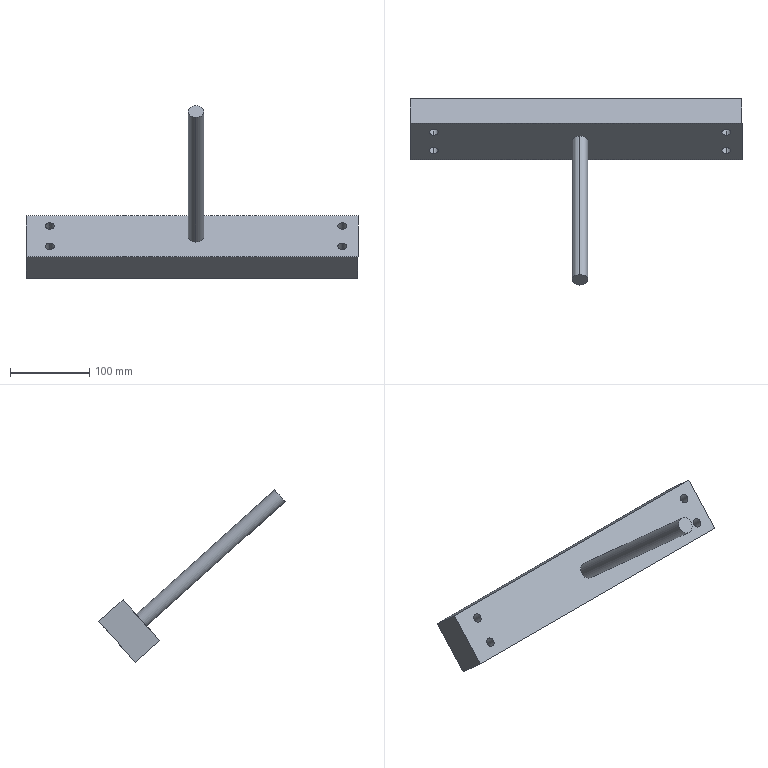Part | Creo | 1 solid | 30 faces | box 418.804 x 235.019 x 217.594 mm | volume 1236938 mm3 | cylinder 18 | plane 12 | commonest cylinder face diameters 11 x8 17.25 x8 20 x2
STEP:
#1=CARTESIAN_POINT('',(0.,0.,0.));
#2=DIRECTION('',(0.,0.,1.));
#3=DIRECTION('',(1.,0.,0.));
#4=AXIS2_PLACEMENT_3D('',#1,#2,#3);
#5=CARTESIAN_POINT('',(5.524,278.128,205.97));
#6=VERTEX_POINT('',#5);
#7=CARTESIAN_POINT('',(5.524,264.758,191.095));
#8=VERTEX_POINT('',#7);
#9=CARTESIAN_POINT('',(5.524,271.443,198.533));
#10=DIRECTION('',(0.000000011,-0.7437,0.6685));
#11=DIRECTION('',(-0.000000021,0.6685,0.7437));
#12=AXIS2_PLACEMENT_3D('',#9,#10,#11);
#13=CIRCLE('',#12,10.);
#14=EDGE_CURVE('',#6,#8,#13,.T.);
#15=ORIENTED_EDGE('',*,*,#14,.F.);
#16=CARTESIAN_POINT('',(5.524,271.443,198.533));
#17=DIRECTION('',(0.000000011,-0.7437,0.6685));
#18=DIRECTION('',(0.,-0.6685,-0.7437));
#19=AXIS2_PLACEMENT_3D('',#16,#17,#18);
#20=CIRCLE('',#19,10.);
#21=EDGE_CURVE('',#8,#6,#20,.T.);
#22=ORIENTED_EDGE('',*,*,#21,.F.);
#23=EDGE_LOOP('',(#15,#22));
#24=FACE_OUTER_BOUND('',#23,.F.);
#25=CARTESIAN_POINT('',(5.524,271.443,198.533));
#26=DIRECTION('',(-0.000000011,0.7437,-0.6685));
#27=DIRECTION('',(0.,0.6685,0.7437));
#28=AXIS2_PLACEMENT_3D('',#25,#26,#27);
#29=PLANE('',#28);
#30=ADVANCED_FACE('',(#24),#29,.F.);
#31=ORIENTED_EDGE('',*,*,#14,.T.);
#32=CARTESIAN_POINT('',(5.524,439.537,34.005));
#33=VERTEX_POINT('',#32);
#34=CARTESIAN_POINT('',(5.524,264.758,191.095));
#35=DIRECTION('',(-0.000000011,0.7437,-0.6685));
#36=VECTOR('',#35,235.);
#37=LINE('',#34,#36);
#38=EDGE_CURVE('',#8,#33,#37,.T.);
#39=ORIENTED_EDGE('',*,*,#38,.T.);
#40=CARTESIAN_POINT('',(5.524,452.906,48.88));
#41=VERTEX_POINT('',#40);
#42=CARTESIAN_POINT('',(5.524,446.222,41.442));
#43=DIRECTION('',(-0.000000011,0.7437,-0.6685));
#44=DIRECTION('',(0.000000021,-0.6685,-0.7437));
#45=AXIS2_PLACEMENT_3D('',#42,#43,#44);
#46=CIRCLE('',#45,10.);
#47=EDGE_CURVE('',#33,#41,#46,.T.);
#48=ORIENTED_EDGE('',*,*,#47,.T.);
#49=CARTESIAN_POINT('',(5.524,278.128,205.97));
#50=DIRECTION('',(-0.000000011,0.7437,-0.6685));
#51=VECTOR('',#50,235.);
#52=LINE('',#49,#51);
#53=EDGE_CURVE('',#6,#41,#52,.T.);
#54=ORIENTED_EDGE('',*,*,#53,.F.);
#55=EDGE_LOOP('',(#31,#39,#48,#54));
#56=FACE_OUTER_BOUND('',#55,.F.);
#57=CARTESIAN_POINT('',(5.524,327.223,148.398));
#58=DIRECTION('',(-0.000000011,0.7437,-0.6685));
#59=DIRECTION('',(0.,0.6685,0.7437));
#60=AXIS2_PLACEMENT_3D('',#57,#58,#59);
#61=CYLINDRICAL_SURFACE('',#60,10.);
#62=ADVANCED_FACE('',(#56),#61,.T.);
#63=ORIENTED_EDGE('',*,*,#21,.T.);
#64=ORIENTED_EDGE('',*,*,#53,.T.);
#65=CARTESIAN_POINT('',(5.524,446.222,41.442));
#66=DIRECTION('',(-0.000000011,0.7437,-0.6685));
#67=DIRECTION('',(-0.000000011,0.6685,0.7437));
#68=AXIS2_PLACEMENT_3D('',#65,#66,#67);
#69=CIRCLE('',#68,10.);
#70=EDGE_CURVE('',#41,#33,#69,.T.);
#71=ORIENTED_EDGE('',*,*,#70,.T.);
#72=ORIENTED_EDGE('',*,*,#38,.F.);
#73=EDGE_LOOP('',(#63,#64,#71,#72));
#74=FACE_OUTER_BOUND('',#73,.F.);
#75=CARTESIAN_POINT('',(5.524,327.223,148.398));
#76=DIRECTION('',(-0.000000011,0.7437,-0.6685));
#77=DIRECTION('',(0.,0.6685,0.7437));
#78=AXIS2_PLACEMENT_3D('',#75,#76,#77);
#79=CYLINDRICAL_SURFACE('',#78,10.);
#80=ADVANCED_FACE('',(#74),#79,.T.);
#81=CARTESIAN_POINT('',(209.927,469.284,67.101));
#82=VERTEX_POINT('',#81);
#83=CARTESIAN_POINT('',(209.927,423.159,15.783));
#84=VERTEX_POINT('',#83);
#85=CARTESIAN_POINT('',(209.927,469.284,67.101));
#86=DIRECTION('',(0.,-0.6685,-0.7437));
#87=VECTOR('',#86,69.);
#88=LINE('',#85,#87);
#89=EDGE_CURVE('',#82,#84,#88,.T.);
#90=ORIENTED_EDGE('',*,*,#89,.T.);
#91=CARTESIAN_POINT('',(-208.878,423.159,15.783));
#92=VERTEX_POINT('',#91);
#93=CARTESIAN_POINT('',(-208.878,423.159,15.783));
#94=DIRECTION('',(1.,0.000000025,0.000000011));
#95=VECTOR('',#94,418.804);
#96=LINE('',#93,#95);
#97=EDGE_CURVE('',#92,#84,#96,.T.);
#98=ORIENTED_EDGE('',*,*,#97,.F.);
#99=CARTESIAN_POINT('',(-208.878,469.284,67.101));
#100=VERTEX_POINT('',#99);
#101=CARTESIAN_POINT('',(-208.878,423.159,15.783));
#102=DIRECTION('',(0.,0.6685,0.7437));
#103=VECTOR('',#102,69.);
#104=LINE('',#101,#103);
#105=EDGE_CURVE('',#92,#100,#104,.T.);
#106=ORIENTED_EDGE('',*,*,#105,.T.);
#107=CARTESIAN_POINT('',(209.927,469.284,67.101));
#108=DIRECTION('',(-1.,-0.000000025,-0.000000011));
#109=VECTOR('',#108,418.804);
#110=LINE('',#107,#109);
#111=EDGE_CURVE('',#82,#100,#110,.T.);
#112=ORIENTED_EDGE('',*,*,#111,.F.);
#113=EDGE_LOOP('',(#90,#98,#106,#112));
#114=FACE_OUTER_BOUND('',#113,.F.);
#115=CARTESIAN_POINT('',(-173.378,457.753,54.272));
#116=VERTEX_POINT('',#115);
#117=CARTESIAN_POINT('',(-178.878,454.076,50.181));
#118=VERTEX_POINT('',#117);
#119=CARTESIAN_POINT('',(-178.878,457.753,54.272));
#120=DIRECTION('',(-0.000000011,0.7437,-0.6685));
#121=DIRECTION('',(1.,0.000000015,0.));
#122=AXIS2_PLACEMENT_3D('',#119,#120,#121);
#123=CIRCLE('',#122,5.5);
#124=EDGE_CURVE('',#116,#118,#123,.T.);
#125=ORIENTED_EDGE('',*,*,#124,.F.);
#126=CARTESIAN_POINT('',(-178.878,461.429,58.362));
#127=VERTEX_POINT('',#126);
#128=CARTESIAN_POINT('',(-178.878,457.753,54.272));
#129=DIRECTION('',(-0.000000011,0.7437,-0.6685));
#130=DIRECTION('',(0.,0.6685,0.7437));
#131=AXIS2_PLACEMENT_3D('',#128,#129,#130);
#132=CIRCLE('',#131,5.5);
#133=EDGE_CURVE('',#127,#116,#132,.T.);
#134=ORIENTED_EDGE('',*,*,#133,.F.);
#135=CARTESIAN_POINT('',(-178.878,457.753,54.272));
#136=DIRECTION('',(-0.000000011,0.7437,-0.6685));
#137=DIRECTION('',(0.,-0.6685,-0.7437));
#138=AXIS2_PLACEMENT_3D('',#135,#136,#137);
#139=CIRCLE('',#138,5.5);
#140=EDGE_CURVE('',#118,#127,#139,.T.);
#141=ORIENTED_EDGE('',*,*,#140,.F.);
#142=EDGE_LOOP('',(#125,#134,#141));
#143=FACE_BOUND('',#142,.F.);
#144=CARTESIAN_POINT('',(195.427,434.691,28.613));
#145=VERTEX_POINT('',#144);
#146=CARTESIAN_POINT('',(189.927,431.014,24.522));
#147=VERTEX_POINT('',#146);
#148=CARTESIAN_POINT('',(189.927,434.691,28.613));
#149=DIRECTION('',(-0.000000011,0.7437,-0.6685));
#150=DIRECTION('',(1.,0.000000015,0.));
#151=AXIS2_PLACEMENT_3D('',#148,#149,#150);
#152=CIRCLE('',#151,5.5);
#153=EDGE_CURVE('',#145,#147,#152,.T.);
#154=ORIENTED_EDGE('',*,*,#153,.F.);
#155=CARTESIAN_POINT('',(189.927,438.367,32.703));
#156=VERTEX_POINT('',#155);
#157=CARTESIAN_POINT('',(189.927,434.691,28.613));
#158=DIRECTION('',(-0.000000011,0.7437,-0.6685));
#159=DIRECTION('',(0.,0.6685,0.7437));
#160=AXIS2_PLACEMENT_3D('',#157,#158,#159);
#161=CIRCLE('',#160,5.5);
#162=EDGE_CURVE('',#156,#145,#161,.T.);
#163=ORIENTED_EDGE('',*,*,#162,.F.);
#164=CARTESIAN_POINT('',(189.927,434.691,28.613));
#165=DIRECTION('',(-0.000000011,0.7437,-0.6685));
#166=DIRECTION('',(0.,-0.6685,-0.7437));
#167=AXIS2_PLACEMENT_3D('',#164,#165,#166);
#168=CIRCLE('',#167,5.5);
#169=EDGE_CURVE('',#147,#156,#168,.T.);
#170=ORIENTED_EDGE('',*,*,#169,.F.);
#171=EDGE_LOOP('',(#154,#163,#170));
#172=FACE_BOUND('',#171,.F.);
#173=CARTESIAN_POINT('',(195.427,457.753,54.272));
#174=VERTEX_POINT('',#173);
#175=CARTESIAN_POINT('',(189.927,454.076,50.181));
#176=VERTEX_POINT('',#175);
#177=CARTESIAN_POINT('',(189.927,457.753,54.272));
#178=DIRECTION('',(-0.000000011,0.7437,-0.6685));
#179=DIRECTION('',(1.,0.000000015,0.));
#180=AXIS2_PLACEMENT_3D('',#177,#178,#179);
#181=CIRCLE('',#180,5.5);
#182=EDGE_CURVE('',#174,#176,#181,.T.);
#183=ORIENTED_EDGE('',*,*,#182,.F.);
#184=CARTESIAN_POINT('',(189.927,461.429,58.362));
#185=VERTEX_POINT('',#184);
#186=CARTESIAN_POINT('',(189.927,457.753,54.272));
#187=DIRECTION('',(-0.000000011,0.7437,-0.6685));
#188=DIRECTION('',(0.,0.6685,0.7437));
#189=AXIS2_PLACEMENT_3D('',#186,#187,#188);
#190=CIRCLE('',#189,5.5);
#191=EDGE_CURVE('',#185,#174,#190,.T.);
#192=ORIENTED_EDGE('',*,*,#191,.F.);
#193=CARTESIAN_POINT('',(189.927,457.753,54.272));
#194=DIRECTION('',(-0.000000011,0.7437,-0.6685));
#195=DIRECTION('',(0.,-0.6685,-0.7437));
#196=AXIS2_PLACEMENT_3D('',#193,#194,#195);
#197=CIRCLE('',#196,5.5);
#198=EDGE_CURVE('',#176,#185,#197,.T.);
#199=ORIENTED_EDGE('',*,*,#198,.F.);
#200=EDGE_LOOP('',(#183,#192,#199));
#201=FACE_BOUND('',#200,.F.);
#202=CARTESIAN_POINT('',(-173.378,434.691,28.613));
#203=VERTEX_POINT('',#202);
#204=CARTESIAN_POINT('',(-178.878,431.014,24.522));
#205=VERTEX_POINT('',#204);
#206=CARTESIAN_POINT('',(-178.878,434.691,28.613));
#207=DIRECTION('',(-0.000000011,0.7437,-0.6685));
#208=DIRECTION('',(1.,0.000000015,0.));
#209=AXIS2_PLACEMENT_3D('',#206,#207,#208);
#210=CIRCLE('',#209,5.5);
#211=EDGE_CURVE('',#203,#205,#210,.T.);
#212=ORIENTED_EDGE('',*,*,#211,.F.);
#213=CARTESIAN_POINT('',(-178.878,438.367,32.703));
#214=VERTEX_POINT('',#213);
#215=CARTESIAN_POINT('',(-178.878,434.691,28.613));
#216=DIRECTION('',(-0.000000011,0.7437,-0.6685));
#217=DIRECTION('',(0.,0.6685,0.7437));
#218=AXIS2_PLACEMENT_3D('',#215,#216,#217);
#219=CIRCLE('',#218,5.5);
#220=EDGE_CURVE('',#214,#203,#219,.T.);
#221=ORIENTED_EDGE('',*,*,#220,.F.);
#222=CARTESIAN_POINT('',(-178.878,434.691,28.613));
#223=DIRECTION('',(-0.000000011,0.7437,-0.6685));
#224=DIRECTION('',(0.,-0.6685,-0.7437));
#225=AXIS2_PLACEMENT_3D('',#222,#223,#224);
#226=CIRCLE('',#225,5.5);
#227=EDGE_CURVE('',#205,#214,#226,.T.);
#228=ORIENTED_EDGE('',*,*,#227,.F.);
#229=EDGE_LOOP('',(#212,#221,#228));
#230=FACE_BOUND('',#229,.F.);
#231=ORIENTED_EDGE('',*,*,#47,.F.);
#232=ORIENTED_EDGE('',*,*,#70,.F.);
#233=EDGE_LOOP('',(#231,#232));
#234=FACE_BOUND('',#233,.F.);
#235=CARTESIAN_POINT('',(-53.476,423.159,15.783));
#236=DIRECTION('',(0.000000011,-0.7437,0.6685));
#237=DIRECTION('',(0.,-0.6685,-0.7437));
#238=AXIS2_PLACEMENT_3D('',#235,#236,#237);
#239=PLANE('',#238);
#240=ADVANCED_FACE('',(#114,#143,#172,#201,#230,#234),#239,.T.);
#241=ORIENTED_EDGE('',*,*,#220,.T.);
#242=ORIENTED_EDGE('',*,*,#211,.T.);
#243=CARTESIAN_POINT('',(-178.878,453.326,4.468));
#244=VERTEX_POINT('',#243);
#245=CARTESIAN_POINT('',(-178.878,453.326,4.468));
#246=DIRECTION('',(0.000000011,-0.7437,0.6685));
#247=VECTOR('',#246,30.);
#248=LINE('',#245,#247);
#249=EDGE_CURVE('',#244,#205,#248,.T.);
#250=ORIENTED_EDGE('',*,*,#249,.F.);
#251=CARTESIAN_POINT('',(-173.378,457.003,8.559));
#252=VERTEX_POINT('',#251);
#253=CARTESIAN_POINT('',(-178.878,457.003,8.559));
#254=DIRECTION('',(0.000000011,-0.7437,0.6685));
#255=DIRECTION('',(0.,-0.6685,-0.7437));
#256=AXIS2_PLACEMENT_3D('',#253,#254,#255);
#257=CIRCLE('',#256,5.5);
#258=EDGE_CURVE('',#244,#252,#257,.T.);
#259=ORIENTED_EDGE('',*,*,#258,.T.);
#260=CARTESIAN_POINT('',(-178.878,460.679,12.649));
#261=VERTEX_POINT('',#260);
#262=CARTESIAN_POINT('',(-178.878,457.003,8.559));
#263=DIRECTION('',(0.000000011,-0.7437,0.6685));
#264=DIRECTION('',(1.,0.000000015,0.));
#265=AXIS2_PLACEMENT_3D('',#262,#263,#264);
#266=CIRCLE('',#265,5.5);
#267=EDGE_CURVE('',#252,#261,#266,.T.);
#268=ORIENTED_EDGE('',*,*,#267,.T.);
#269=CARTESIAN_POINT('',(-178.878,460.679,12.649));
#270=DIRECTION('',(0.000000011,-0.7437,0.6685));
#271=VECTOR('',#270,30.);
#272=LINE('',#269,#271);
#273=EDGE_CURVE('',#261,#214,#272,.T.);
#274=ORIENTED_EDGE('',*,*,#273,.T.);
#275=EDGE_LOOP('',(#241,#242,#250,#259,#268,#274));
#276=FACE_OUTER_BOUND('',#275,.F.);
#277=CARTESIAN_POINT('',(-178.878,457.003,8.559));
#278=DIRECTION('',(0.000000011,-0.7437,0.6685));
#279=DIRECTION('',(0.,-0.6685,-0.7437));
#280=AXIS2_PLACEMENT_3D('',#277,#278,#279);
#281=CYLINDRICAL_SURFACE('',#280,5.5);
#282=ADVANCED_FACE('',(#276),#281,.F.);
#283=ORIENTED_EDGE('',*,*,#227,.T.);
#284=ORIENTED_EDGE('',*,*,#273,.F.);
#285=CARTESIAN_POINT('',(-184.378,457.003,8.559));
#286=VERTEX_POINT('',#285);
#287=CARTESIAN_POINT('',(-178.878,457.003,8.559));
#288=DIRECTION('',(0.000000011,-0.7437,0.6685));
#289=DIRECTION('',(0.,0.6685,0.7437));
#290=AXIS2_PLACEMENT_3D('',#287,#288,#289);
#291=CIRCLE('',#290,5.5);
#292=EDGE_CURVE('',#261,#286,#291,.T.);
#293=ORIENTED_EDGE('',*,*,#292,.T.);
#294=CARTESIAN_POINT('',(-178.878,457.003,8.559));
#295=DIRECTION('',(0.000000011,-0.7437,0.6685));
#296=DIRECTION('',(-1.,-0.000000015,0.));
#297=AXIS2_PLACEMENT_3D('',#294,#295,#296);
#298=CIRCLE('',#297,5.5);
#299=EDGE_CURVE('',#286,#244,#298,.T.);
#300=ORIENTED_EDGE('',*,*,#299,.T.);
#301=ORIENTED_EDGE('',*,*,#249,.T.);
#302=EDGE_LOOP('',(#283,#284,#293,#300,#301));
#303=FACE_OUTER_BOUND('',#302,.F.);
#304=CARTESIAN_POINT('',(-178.878,457.003,8.559));
#305=DIRECTION('',(0.000000011,-0.7437,0.6685));
#306=DIRECTION('',(0.,-0.6685,-0.7437));
#307=AXIS2_PLACEMENT_3D('',#304,#305,#306);
#308=CYLINDRICAL_SURFACE('',#307,5.5);
#309=ADVANCED_FACE('',(#303),#308,.F.);
#310=CARTESIAN_POINT('',(-187.503,457.003,8.559));
#311=VERTEX_POINT('',#310);
#312=CARTESIAN_POINT('',(-178.878,462.768,14.973));
#313=VERTEX_POINT('',#312);
#314=CARTESIAN_POINT('',(-178.878,457.003,8.559));
#315=DIRECTION('',(-0.000000011,0.7437,-0.6685));
#316=DIRECTION('',(-1.,-0.000000015,0.));
#317=AXIS2_PLACEMENT_3D('',#314,#315,#316);
#318=CIRCLE('',#317,8.625);
#319=EDGE_CURVE('',#311,#313,#318,.T.);
#320=ORIENTED_EDGE('',*,*,#319,.F.);
#321=CARTESIAN_POINT('',(-178.878,451.237,2.144));
#322=VERTEX_POINT('',#321);
#323=CARTESIAN_POINT('',(-178.878,457.003,8.559));
#324=DIRECTION('',(-0.000000011,0.7437,-0.6685));
#325=DIRECTION('',(0.,-0.6685,-0.7437));
#326=AXIS2_PLACEMENT_3D('',#323,#324,#325);
#327=CIRCLE('',#326,8.625);
#328=EDGE_CURVE('',#322,#311,#327,.T.);
#329=ORIENTED_EDGE('',*,*,#328,.F.);
#330=CARTESIAN_POINT('',(-170.253,457.003,8.559));
#331=VERTEX_POINT('',#330);
#332=CARTESIAN_POINT('',(-178.878,457.003,8.559));
#333=DIRECTION('',(-0.000000011,0.7437,-0.6685));
#334=DIRECTION('',(1.,0.000000015,0.));
#335=AXIS2_PLACEMENT_3D('',#332,#333,#334);
#336=CIRCLE('',#335,8.625);
#337=EDGE_CURVE('',#331,#322,#336,.T.);
#338=ORIENTED_EDGE('',*,*,#337,.F.);
#339=CARTESIAN_POINT('',(-178.878,457.003,8.559));
#340=DIRECTION('',(-0.000000011,0.7437,-0.6685));
#341=DIRECTION('',(0.,0.6685,0.7437));
#342=AXIS2_PLACEMENT_3D('',#339,#340,#341);
#343=CIRCLE('',#342,8.625);
#344=EDGE_CURVE('',#313,#331,#343,.T.);
#345=ORIENTED_EDGE('',*,*,#344,.F.);
#346=EDGE_LOOP('',(#320,#329,#338,#345));
#347=FACE_OUTER_BOUND('',#346,.F.);
#348=ORIENTED_EDGE('',*,*,#267,.F.);
#349=ORIENTED_EDGE('',*,*,#258,.F.);
#350=ORIENTED_EDGE('',*,*,#299,.F.);
#351=ORIENTED_EDGE('',*,*,#292,.F.);
#352=EDGE_LOOP('',(#348,#349,#350,#351));
#353=FACE_BOUND('',#352,.F.);
#354=CARTESIAN_POINT('',(-178.878,457.003,8.559));
#355=DIRECTION('',(0.000000011,-0.7437,0.6685));
#356=DIRECTION('',(0.,-0.6685,-0.7437));
#357=AXIS2_PLACEMENT_3D('',#354,#355,#356);
#358=PLANE('',#357);
#359=ADVANCED_FACE('',(#347,#353),#358,.F.);
#360=CARTESIAN_POINT('',(-178.878,470.949,7.62));
#361=VERTEX_POINT('',#360);
#362=CARTESIAN_POINT('',(-187.503,465.184,1.206));
#363=VERTEX_POINT('',#362);
#364=CARTESIAN_POINT('',(-178.878,465.184,1.206));
#365=DIRECTION('',(0.000000011,-0.7437,0.6685));
#366=DIRECTION('',(0.,0.6685,0.7437));
#367=AXIS2_PLACEMENT_3D('',#364,#365,#366);
#368=CIRCLE('',#367,8.625);
#369=EDGE_CURVE('',#361,#363,#368,.T.);
#370=ORIENTED_EDGE('',*,*,#369,.T.);
#371=CARTESIAN_POINT('',(-178.878,459.418,-5.209));
#372=VERTEX_POINT('',#371);
#373=CARTESIAN_POINT('',(-178.878,465.184,1.206));
#374=DIRECTION('',(0.000000011,-0.7437,0.6685));
#375=DIRECTION('',(-1.,-0.000000015,0.));
#376=AXIS2_PLACEMENT_3D('',#373,#374,#375);
#377=CIRCLE('',#376,8.625);
#378=EDGE_CURVE('',#363,#372,#377,.T.);
#379=ORIENTED_EDGE('',*,*,#378,.T.);
#380=CARTESIAN_POINT('',(-178.878,451.237,2.144));
#381=DIRECTION('',(-0.000000011,0.7437,-0.6685));
#382=VECTOR('',#381,11.);
#383=LINE('',#380,#382);
#384=EDGE_CURVE('',#322,#372,#383,.T.);
#385=ORIENTED_EDGE('',*,*,#384,.F.);
#386=ORIENTED_EDGE('',*,*,#328,.T.);
#387=ORIENTED_EDGE('',*,*,#319,.T.);
#388=CARTESIAN_POINT('',(-178.878,462.768,14.973));
#389=DIRECTION('',(-0.000000011,0.7437,-0.6685));
#390=VECTOR('',#389,11.);
#391=LINE('',#388,#390);
#392=EDGE_CURVE('',#313,#361,#391,.T.);
#393=ORIENTED_EDGE('',*,*,#392,.T.);
#394=EDGE_LOOP('',(#370,#379,#385,#386,#387,#393));
#395=FACE_OUTER_BOUND('',#394,.F.);
#396=CARTESIAN_POINT('',(-178.878,457.003,8.559));
#397=DIRECTION('',(-0.000000011,0.7437,-0.6685));
#398=DIRECTION('',(0.,0.6685,0.7437));
#399=AXIS2_PLACEMENT_3D('',#396,#397,#398);
#400=CYLINDRICAL_SURFACE('',#399,8.625);
#401=ADVANCED_FACE('',(#395),#400,.F.);
#402=CARTESIAN_POINT('',(209.927,499.777,39.694));
#403=VERTEX_POINT('',#402);
#404=CARTESIAN_POINT('',(-208.878,499.777,39.694));
#405=VERTEX_POINT('',#404);
#406=CARTESIAN_POINT('',(209.927,499.777,39.694));
#407=DIRECTION('',(-1.,-0.000000025,-0.000000011));
#408=VECTOR('',#407,418.804);
#409=LINE('',#406,#408);
#410=EDGE_CURVE('',#403,#405,#409,.T.);
#411=ORIENTED_EDGE('',*,*,#410,.T.);
#412=CARTESIAN_POINT('',(-208.878,453.653,-11.624));
#413=VERTEX_POINT('',#412);
#414=CARTESIAN_POINT('',(-208.878,499.777,39.694));
#415=DIRECTION('',(0.,-0.6685,-0.7437));
#416=VECTOR('',#415,69.);
#417=LINE('',#414,#416);
#418=EDGE_CURVE('',#405,#413,#417,.T.);
#419=ORIENTED_EDGE('',*,*,#418,.T.);
#420=CARTESIAN_POINT('',(209.927,453.653,-11.624));
#421=VERTEX_POINT('',#420);
#422=CARTESIAN_POINT('',(-208.878,453.653,-11.624));
#423=DIRECTION('',(1.,0.000000025,0.000000011));
#424=VECTOR('',#423,418.804);
#425=LINE('',#422,#424);
#426=EDGE_CURVE('',#413,#421,#425,.T.);
#427=ORIENTED_EDGE('',*,*,#426,.T.);
#428=CARTESIAN_POINT('',(209.927,453.653,-11.624));
#429=DIRECTION('',(0.,0.6685,0.7437));
#430=VECTOR('',#429,69.);
#431=LINE('',#428,#430);
#432=EDGE_CURVE('',#421,#403,#431,.T.);
#433=ORIENTED_EDGE('',*,*,#432,.T.);
#434=EDGE_LOOP('',(#411,#419,#427,#433));
#435=FACE_OUTER_BOUND('',#434,.F.);
#436=CARTESIAN_POINT('',(181.302,488.246,26.865));
#437=VERTEX_POINT('',#436);
#438=CARTESIAN_POINT('',(189.927,482.481,20.45));
#439=VERTEX_POINT('',#438);
#440=CARTESIAN_POINT('',(189.927,488.246,26.865));
#441=DIRECTION('',(0.000000011,-0.7437,0.6685));
#442=DIRECTION('',(-1.,-0.000000015,0.));
#443=AXIS2_PLACEMENT_3D('',#440,#441,#442);
#444=CIRCLE('',#443,8.625);
#445=EDGE_CURVE('',#437,#439,#444,.T.);
#446=ORIENTED_EDGE('',*,*,#445,.F.);
#447=CARTESIAN_POINT('',(189.927,494.012,33.279));
#448=VERTEX_POINT('',#447);
#449=CARTESIAN_POINT('',(189.927,488.246,26.865));
#450=DIRECTION('',(0.000000011,-0.7437,0.6685));
#451=DIRECTION('',(0.,0.6685,0.7437));
#452=AXIS2_PLACEMENT_3D('',#449,#450,#451);
#453=CIRCLE('',#452,8.625);
#454=EDGE_CURVE('',#448,#437,#453,.T.);
#455=ORIENTED_EDGE('',*,*,#454,.F.);
#456=CARTESIAN_POINT('',(189.927,488.246,26.865));
#457=DIRECTION('',(0.000000011,-0.7437,0.6685));
#458=DIRECTION('',(0.,-0.6685,-0.7437));
#459=AXIS2_PLACEMENT_3D('',#456,#457,#458);
#460=CIRCLE('',#459,8.625);
#461=EDGE_CURVE('',#439,#448,#460,.T.);
#462=ORIENTED_EDGE('',*,*,#461,.F.);
#463=EDGE_LOOP('',(#446,#455,#462));
#464=FACE_BOUND('',#463,.F.);
#465=CARTESIAN_POINT('',(30.024,454.99,-10.137));
#466=VERTEX_POINT('',#465);
#467=CARTESIAN_POINT('',(-18.976,454.99,-10.137));
#468=VERTEX_POINT('',#467);
#469=CARTESIAN_POINT('',(30.024,454.99,-10.137));
#470=DIRECTION('',(-1.,-0.000000021,-0.000000007));
#471=VECTOR('',#470,49.);
#472=LINE('',#469,#471);
#473=EDGE_CURVE('',#466,#468,#472,.T.);
#474=ORIENTED_EDGE('',*,*,#473,.T.);
#475=CARTESIAN_POINT('',(-26.976,460.337,-4.187));
#476=VERTEX_POINT('',#475);
#477=CARTESIAN_POINT('',(-18.976,454.99,-10.137));
#478=CARTESIAN_POINT('',(-19.692,454.992,-10.134));
#479=CARTESIAN_POINT('',(-21.07,455.113,-10.));
#480=CARTESIAN_POINT('',(-23.028,455.655,-9.396));
#481=CARTESIAN_POINT('',(-24.696,456.513,-8.442));
#482=CARTESIAN_POINT('',(-25.98,457.629,-7.201));
#483=CARTESIAN_POINT('',(-26.792,458.938,-5.744));
#484=CARTESIAN_POINT('',(-26.972,459.858,-4.72));
#485=CARTESIAN_POINT('',(-26.976,460.337,-4.187));
#486=B_SPLINE_CURVE_WITH_KNOTS('',3,(#477,#478,#479,#480,#481,#482,#483,#484,#485),.UNSPECIFIED.,.F.,.F.,(4,1,1,1,1,1,4),(0.,0.1667,0.3333,0.5,0.6667,0.8333,1.),.UNSPECIFIED.);
#487=EDGE_CURVE('',#468,#476,#486,.T.);
#488=ORIENTED_EDGE('',*,*,#487,.T.);
#489=CARTESIAN_POINT('',(-26.976,493.092,32.257));
#490=VERTEX_POINT('',#489);
#491=CARTESIAN_POINT('',(-26.976,460.337,-4.187));
#492=DIRECTION('',(-0.000000019,0.6685,0.7437));
#493=VECTOR('',#492,49.);
#494=LINE('',#491,#493);
#495=EDGE_CURVE('',#476,#490,#494,.T.);
#496=ORIENTED_EDGE('',*,*,#495,.T.);
#497=CARTESIAN_POINT('',(-18.976,498.44,38.207));
#498=VERTEX_POINT('',#497);
#499=CARTESIAN_POINT('',(-26.972,493.572,32.79));
#500=CARTESIAN_POINT('',(-26.792,494.492,33.814));
#501=CARTESIAN_POINT('',(-25.98,495.801,35.27));
#502=CARTESIAN_POINT('',(-24.697,496.917,36.511));
#503=CARTESIAN_POINT('',(-23.028,497.775,37.466));
#504=CARTESIAN_POINT('',(-21.07,498.317,38.07));
#505=CARTESIAN_POINT('',(-19.692,498.438,38.204));
#506=CARTESIAN_POINT('',(-18.976,498.44,38.207));
#507=B_SPLINE_CURVE_WITH_KNOTS('',3,(#489,#499,#500,#501,#502,#503,#504,#505,#506),.UNSPECIFIED.,.F.,.F.,(4,1,1,1,1,1,4),(0.,0.1667,0.3333,0.5,0.6667,0.8333,1.),.UNSPECIFIED.);
#508=EDGE_CURVE('',#490,#498,#507,.T.);
#509=ORIENTED_EDGE('',*,*,#508,.T.);
#510=CARTESIAN_POINT('',(30.024,498.44,38.207));
#511=VERTEX_POINT('',#510);
#512=CARTESIAN_POINT('',(-18.976,498.44,38.207));
#513=DIRECTION('',(1.,0.000000021,0.000000007));
#514=VECTOR('',#513,49.);
#515=LINE('',#512,#514);
#516=EDGE_CURVE('',#498,#511,#515,.T.);
#517=ORIENTED_EDGE('',*,*,#516,.T.);
#518=CARTESIAN_POINT('',(38.024,493.092,32.257));
#519=VERTEX_POINT('',#518);
#520=CARTESIAN_POINT('',(30.741,498.438,38.204));
#521=CARTESIAN_POINT('',(32.118,498.317,38.07));
#522=CARTESIAN_POINT('',(34.077,497.775,37.466));
#523=CARTESIAN_POINT('',(35.745,496.917,36.512));
#524=CARTESIAN_POINT('',(37.029,495.801,35.271));
#525=CARTESIAN_POINT('',(37.841,494.492,33.814));
#526=CARTESIAN_POINT('',(38.021,493.572,32.79));
#527=CARTESIAN_POINT('',(38.024,493.092,32.257));
#528=B_SPLINE_CURVE_WITH_KNOTS('',3,(#510,#520,#521,#522,#523,#524,#525,#526,#527),.UNSPECIFIED.,.F.,.F.,(4,1,1,1,1,1,4),(0.,0.1667,0.3333,0.5,0.6667,0.8333,1.),.UNSPECIFIED.);
#529=EDGE_CURVE('',#511,#519,#528,.T.);
#530=ORIENTED_EDGE('',*,*,#529,.T.);
#531=CARTESIAN_POINT('',(38.024,460.337,-4.187));
#532=VERTEX_POINT('',#531);
#533=CARTESIAN_POINT('',(38.024,493.092,32.257));
#534=DIRECTION('',(0.000000013,-0.6685,-0.7437));
#535=VECTOR('',#534,49.);
#536=LINE('',#533,#535);
#537=EDGE_CURVE('',#519,#532,#536,.T.);
#538=ORIENTED_EDGE('',*,*,#537,.T.);
#539=CARTESIAN_POINT('',(38.021,459.858,-4.72));
#540=CARTESIAN_POINT('',(37.841,458.938,-5.744));
#541=CARTESIAN_POINT('',(37.029,457.629,-7.2));
#542=CARTESIAN_POINT('',(35.746,456.513,-8.441));
#543=CARTESIAN_POINT('',(34.077,455.655,-9.396));
#544=CARTESIAN_POINT('',(32.119,455.113,-10.));
#545=CARTESIAN_POINT('',(30.741,454.992,-10.134));
#546=CARTESIAN_POINT('',(30.024,454.99,-10.137));
#547=B_SPLINE_CURVE_WITH_KNOTS('',3,(#531,#539,#540,#541,#542,#543,#544,#545,#546),.UNSPECIFIED.,.F.,.F.,(4,1,1,1,1,1,4),(0.,0.1667,0.3333,0.5,0.6667,0.8333,1.),.UNSPECIFIED.);
#548=EDGE_CURVE('',#532,#466,#547,.T.);
#549=ORIENTED_EDGE('',*,*,#548,.T.);
#550=EDGE_LOOP('',(#474,#488,#496,#509,#517,#530,#538,#549));
#551=FACE_BOUND('',#550,.F.);
#552=CARTESIAN_POINT('',(-187.503,488.246,26.865));
#553=VERTEX_POINT('',#552);
#554=CARTESIAN_POINT('',(-178.878,482.481,20.45));
#555=VERTEX_POINT('',#554);
#556=CARTESIAN_POINT('',(-178.878,488.246,26.865));
#557=DIRECTION('',(0.000000011,-0.7437,0.6685));
#558=DIRECTION('',(-1.,-0.000000015,0.));
#559=AXIS2_PLACEMENT_3D('',#556,#557,#558);
#560=CIRCLE('',#559,8.625);
#561=EDGE_CURVE('',#553,#555,#560,.T.);
#562=ORIENTED_EDGE('',*,*,#561,.F.);
#563=CARTESIAN_POINT('',(-178.878,494.012,33.279));
#564=VERTEX_POINT('',#563);
#565=CARTESIAN_POINT('',(-178.878,488.246,26.865));
#566=DIRECTION('',(0.000000011,-0.7437,0.6685));
#567=DIRECTION('',(0.,0.6685,0.7437));
#568=AXIS2_PLACEMENT_3D('',#565,#566,#567);
#569=CIRCLE('',#568,8.625);
#570=EDGE_CURVE('',#564,#553,#569,.T.);
#571=ORIENTED_EDGE('',*,*,#570,.F.);
#572=CARTESIAN_POINT('',(-178.878,488.246,26.865));
#573=DIRECTION('',(0.000000011,-0.7437,0.6685));
#574=DIRECTION('',(0.,-0.6685,-0.7437));
#575=AXIS2_PLACEMENT_3D('',#572,#573,#574);
#576=CIRCLE('',#575,8.625);
#577=EDGE_CURVE('',#555,#564,#576,.T.);
#578=ORIENTED_EDGE('',*,*,#577,.F.);
#579=EDGE_LOOP('',(#562,#571,#578));
#580=FACE_BOUND('',#579,.F.);
#581=CARTESIAN_POINT('',(181.302,465.184,1.206));
#582=VERTEX_POINT('',#581);
#583=CARTESIAN_POINT('',(189.927,459.418,-5.209));
#584=VERTEX_POINT('',#583);
#585=CARTESIAN_POINT('',(189.927,465.184,1.206));
#586=DIRECTION('',(0.000000011,-0.7437,0.6685));
#587=DIRECTION('',(-1.,-0.000000015,0.));
#588=AXIS2_PLACEMENT_3D('',#585,#586,#587);
#589=CIRCLE('',#588,8.625);
#590=EDGE_CURVE('',#582,#584,#589,.T.);
#591=ORIENTED_EDGE('',*,*,#590,.F.);
#592=CARTESIAN_POINT('',(189.927,470.949,7.62));
#593=VERTEX_POINT('',#592);
#594=CARTESIAN_POINT('',(189.927,465.184,1.206));
#595=DIRECTION('',(0.000000011,-0.7437,0.6685));
#596=DIRECTION('',(0.,0.6685,0.7437));
#597=AXIS2_PLACEMENT_3D('',#594,#595,#596);
#598=CIRCLE('',#597,8.625);
#599=EDGE_CURVE('',#593,#582,#598,.T.);
#600=ORIENTED_EDGE('',*,*,#599,.F.);
#601=CARTESIAN_POINT('',(189.927,465.184,1.206));
#602=DIRECTION('',(0.000000011,-0.7437,0.6685));
#603=DIRECTION('',(0.,-0.6685,-0.7437));
#604=AXIS2_PLACEMENT_3D('',#601,#602,#603);
#605=CIRCLE('',#604,8.625);
#606=EDGE_CURVE('',#584,#593,#605,.T.);
#607=ORIENTED_EDGE('',*,*,#606,.F.);
#608=EDGE_LOOP('',(#591,#600,#607));
#609=FACE_BOUND('',#608,.F.);
#610=ORIENTED_EDGE('',*,*,#378,.F.);
#611=ORIENTED_EDGE('',*,*,#369,.F.);
#612=CARTESIAN_POINT('',(-178.878,465.184,1.206));
#613=DIRECTION('',(0.000000011,-0.7437,0.6685));
#614=DIRECTION('',(0.,-0.6685,-0.7437));
#615=AXIS2_PLACEMENT_3D('',#612,#613,#614);
#616=CIRCLE('',#615,8.625);
#617=EDGE_CURVE('',#372,#361,#616,.T.);
#618=ORIENTED_EDGE('',*,*,#617,.F.);
#619=EDGE_LOOP('',(#610,#611,#618));
#620=FACE_BOUND('',#619,.F.);
#621=CARTESIAN_POINT('',(-53.476,453.653,-11.624));
#622=DIRECTION('',(0.000000011,-0.7437,0.6685));
#623=DIRECTION('',(0.,-0.6685,-0.7437));
#624=AXIS2_PLACEMENT_3D('',#621,#622,#623);
#625=PLANE('',#624);
#626=ADVANCED_FACE('',(#435,#464,#551,#580,#609,#620),#625,.F.);
#627=ORIENTED_EDGE('',*,*,#570,.T.);
#628=ORIENTED_EDGE('',*,*,#561,.T.);
#629=CARTESIAN_POINT('',(-178.878,474.299,27.803));
#630=VERTEX_POINT('',#629);
#631=CARTESIAN_POINT('',(-178.878,474.299,27.803));
#632=DIRECTION('',(-0.000000011,0.7437,-0.6685));
#633=VECTOR('',#632,11.);
#634=LINE('',#631,#633);
#635=EDGE_CURVE('',#630,#555,#634,.T.);
#636=ORIENTED_EDGE('',*,*,#635,.F.);
#637=CARTESIAN_POINT('',(-187.503,480.065,34.218));
#638=VERTEX_POINT('',#637);
#639=CARTESIAN_POINT('',(-178.878,480.065,34.218));
#640=DIRECTION('',(-0.000000011,0.7437,-0.6685));
#641=DIRECTION('',(0.,-0.6685,-0.7437));
#642=AXIS2_PLACEMENT_3D('',#639,#640,#641);
#643=CIRCLE('',#642,8.625);
#644=EDGE_CURVE('',#630,#638,#643,.T.);
#645=ORIENTED_EDGE('',*,*,#644,.T.);
#646=CARTESIAN_POINT('',(-178.878,485.831,40.632));
#647=VERTEX_POINT('',#646);
#648=CARTESIAN_POINT('',(-178.878,480.065,34.218));
#649=DIRECTION('',(-0.000000011,0.7437,-0.6685));
#650=DIRECTION('',(-1.,-0.000000015,0.));
#651=AXIS2_PLACEMENT_3D('',#648,#649,#650);
#652=CIRCLE('',#651,8.625);
#653=EDGE_CURVE('',#638,#647,#652,.T.);
#654=ORIENTED_EDGE('',*,*,#653,.T.);
#655=CARTESIAN_POINT('',(-178.878,485.831,40.632));
#656=DIRECTION('',(-0.000000011,0.7437,-0.6685));
#657=VECTOR('',#656,11.);
#658=LINE('',#655,#657);
#659=EDGE_CURVE('',#647,#564,#658,.T.);
#660=ORIENTED_EDGE('',*,*,#659,.T.);
#661=EDGE_LOOP('',(#627,#628,#636,#645,#654,#660));
#662=FACE_OUTER_BOUND('',#661,.F.);
#663=CARTESIAN_POINT('',(-178.878,480.065,34.218));
#664=DIRECTION('',(-0.000000011,0.7437,-0.6685));
#665=DIRECTION('',(0.,0.6685,0.7437));
#666=AXIS2_PLACEMENT_3D('',#663,#664,#665);
#667=CYLINDRICAL_SURFACE('',#666,8.625);
#668=ADVANCED_FACE('',(#662),#667,.F.);
#669=ORIENTED_EDGE('',*,*,#577,.T.);
#670=ORIENTED_EDGE('',*,*,#659,.F.);
#671=CARTESIAN_POINT('',(-170.253,480.065,34.218));
#672=VERTEX_POINT('',#671);
#673=CARTESIAN_POINT('',(-178.878,480.065,34.218));
#674=DIRECTION('',(-0.000000011,0.7437,-0.6685));
#675=DIRECTION('',(0.,0.6685,0.7437));
#676=AXIS2_PLACEMENT_3D('',#673,#674,#675);
#677=CIRCLE('',#676,8.625);
#678=EDGE_CURVE('',#647,#672,#677,.T.);
#679=ORIENTED_EDGE('',*,*,#678,.T.);
#680=CARTESIAN_POINT('',(-178.878,480.065,34.218));
#681=DIRECTION('',(-0.000000011,0.7437,-0.6685));
#682=DIRECTION('',(1.,0.000000015,0.));
#683=AXIS2_PLACEMENT_3D('',#680,#681,#682);
#684=CIRCLE('',#683,8.625);
#685=EDGE_CURVE('',#672,#630,#684,.T.);
#686=ORIENTED_EDGE('',*,*,#685,.T.);
#687=ORIENTED_EDGE('',*,*,#635,.T.);
#688=EDGE_LOOP('',(#669,#670,#679,#686,#687));
#689=FACE_OUTER_BOUND('',#688,.F.);
#690=CARTESIAN_POINT('',(-178.878,480.065,34.218));
#691=DIRECTION('',(-0.000000011,0.7437,-0.6685));
#692=DIRECTION('',(0.,0.6685,0.7437));
#693=AXIS2_PLACEMENT_3D('',#690,#691,#692);
#694=CYLINDRICAL_SURFACE('',#693,8.625);
#695=ADVANCED_FACE('',(#689),#694,.F.);
#696=ORIENTED_EDGE('',*,*,#653,.F.);
#697=ORIENTED_EDGE('',*,*,#644,.F.);
#698=ORIENTED_EDGE('',*,*,#685,.F.);
#699=ORIENTED_EDGE('',*,*,#678,.F.);
#700=EDGE_LOOP('',(#696,#697,#698,#699));
#701=FACE_OUTER_BOUND('',#700,.F.);
#702=CARTESIAN_POINT('',(-173.378,480.065,34.218));
#703=VERTEX_POINT('',#702);
#704=CARTESIAN_POINT('',(-178.878,483.742,38.308));
#705=VERTEX_POINT('',#704);
#706=CARTESIAN_POINT('',(-178.878,480.065,34.218));
#707=DIRECTION('',(0.000000011,-0.7437,0.6685));
#708=DIRECTION('',(1.,0.000000015,0.));
#709=AXIS2_PLACEMENT_3D('',#706,#707,#708);
#710=CIRCLE('',#709,5.5);
#711=EDGE_CURVE('',#703,#705,#710,.T.);
#712=ORIENTED_EDGE('',*,*,#711,.F.);
#713=CARTESIAN_POINT('',(-178.878,476.388,30.127));
#714=VERTEX_POINT('',#713);
#715=CARTESIAN_POINT('',(-178.878,480.065,34.218));
#716=DIRECTION('',(0.000000011,-0.7437,0.6685));
#717=DIRECTION('',(0.,-0.6685,-0.7437));
#718=AXIS2_PLACEMENT_3D('',#715,#716,#717);
#719=CIRCLE('',#718,5.5);
#720=EDGE_CURVE('',#714,#703,#719,.T.);
#721=ORIENTED_EDGE('',*,*,#720,.F.);
#722=CARTESIAN_POINT('',(-184.378,480.065,34.218));
#723=VERTEX_POINT('',#722);
#724=CARTESIAN_POINT('',(-178.878,480.065,34.218));
#725=DIRECTION('',(0.000000011,-0.7437,0.6685));
#726=DIRECTION('',(-1.,-0.000000015,0.));
#727=AXIS2_PLACEMENT_3D('',#724,#725,#726);
#728=CIRCLE('',#727,5.5);
#729=EDGE_CURVE('',#723,#714,#728,.T.);
#730=ORIENTED_EDGE('',*,*,#729,.F.);
#731=CARTESIAN_POINT('',(-178.878,480.065,34.218));
#732=DIRECTION('',(0.000000011,-0.7437,0.6685));
#733=DIRECTION('',(0.,0.6685,0.7437));
#734=AXIS2_PLACEMENT_3D('',#731,#732,#733);
#735=CIRCLE('',#734,5.5);
#736=EDGE_CURVE('',#705,#723,#735,.T.);
#737=ORIENTED_EDGE('',*,*,#736,.F.);
#738=EDGE_LOOP('',(#712,#721,#730,#737));
#739=FACE_BOUND('',#738,.F.);
#740=CARTESIAN_POINT('',(-178.878,480.065,34.218));
#741=DIRECTION('',(0.000000011,-0.7437,0.6685));
#742=DIRECTION('',(0.,-0.6685,-0.7437));
#743=AXIS2_PLACEMENT_3D('',#740,#741,#742);
#744=PLANE('',#743);
#745=ADVANCED_FACE('',(#701,#739),#744,.F.);
#746=ORIENTED_EDGE('',*,*,#133,.T.);
#747=ORIENTED_EDGE('',*,*,#124,.T.);
#748=CARTESIAN_POINT('',(-178.878,476.388,30.127));
#749=DIRECTION('',(0.000000011,-0.7437,0.6685));
#750=VECTOR('',#749,30.);
#751=LINE('',#748,#750);
#752=EDGE_CURVE('',#714,#118,#751,.T.);
#753=ORIENTED_EDGE('',*,*,#752,.F.);
#754=ORIENTED_EDGE('',*,*,#720,.T.);
#755=ORIENTED_EDGE('',*,*,#711,.T.);
#756=CARTESIAN_POINT('',(-178.878,483.742,38.308));
#757=DIRECTION('',(0.000000011,-0.7437,0.6685));
#758=VECTOR('',#757,30.);
#759=LINE('',#756,#758);
#760=EDGE_CURVE('',#705,#127,#759,.T.);
#761=ORIENTED_EDGE('',*,*,#760,.T.);
#762=EDGE_LOOP('',(#746,#747,#753,#754,#755,#761));
#763=FACE_OUTER_BOUND('',#762,.F.);
#764=CARTESIAN_POINT('',(-178.878,480.065,34.218));
#765=DIRECTION('',(0.000000011,-0.7437,0.6685));
#766=DIRECTION('',(0.,-0.6685,-0.7437));
#767=AXIS2_PLACEMENT_3D('',#764,#765,#766);
#768=CYLINDRICAL_SURFACE('',#767,5.5);
#769=ADVANCED_FACE('',(#763),#768,.F.);
#770=ORIENTED_EDGE('',*,*,#140,.T.);
#771=ORIENTED_EDGE('',*,*,#760,.F.);
#772=ORIENTED_EDGE('',*,*,#736,.T.);
#773=ORIENTED_EDGE('',*,*,#729,.T.);
#774=ORIENTED_EDGE('',*,*,#752,.T.);
#775=EDGE_LOOP('',(#770,#771,#772,#773,#774));
#776=FACE_OUTER_BOUND('',#775,.F.);
#777=CARTESIAN_POINT('',(-178.878,480.065,34.218));
#778=DIRECTION('',(0.000000011,-0.7437,0.6685));
#779=DIRECTION('',(0.,-0.6685,-0.7437));
#780=AXIS2_PLACEMENT_3D('',#777,#778,#779);
#781=CYLINDRICAL_SURFACE('',#780,5.5);
#782=ADVANCED_FACE('',(#776),#781,.F.);
#783=ORIENTED_EDGE('',*,*,#454,.T.);
#784=ORIENTED_EDGE('',*,*,#445,.T.);
#785=CARTESIAN_POINT('',(189.927,474.299,27.803));
#786=VERTEX_POINT('',#785);
#787=CARTESIAN_POINT('',(189.927,474.299,27.803));
#788=DIRECTION('',(-0.000000011,0.7437,-0.6685));
#789=VECTOR('',#788,11.);
#790=LINE('',#787,#789);
#791=EDGE_CURVE('',#786,#439,#790,.T.);
#792=ORIENTED_EDGE('',*,*,#791,.F.);
#793=CARTESIAN_POINT('',(181.302,480.065,34.218));
#794=VERTEX_POINT('',#793);
#795=CARTESIAN_POINT('',(189.927,480.065,34.218));
#796=DIRECTION('',(-0.000000011,0.7437,-0.6685));
#797=DIRECTION('',(0.,-0.6685,-0.7437));
#798=AXIS2_PLACEMENT_3D('',#795,#796,#797);
#799=CIRCLE('',#798,8.625);
#800=EDGE_CURVE('',#786,#794,#799,.T.);
#801=ORIENTED_EDGE('',*,*,#800,.T.);
#802=CARTESIAN_POINT('',(189.927,485.831,40.632));
#803=VERTEX_POINT('',#802);
#804=CARTESIAN_POINT('',(189.927,480.065,34.218));
#805=DIRECTION('',(-0.000000011,0.7437,-0.6685));
#806=DIRECTION('',(-1.,-0.000000015,0.));
#807=AXIS2_PLACEMENT_3D('',#804,#805,#806);
#808=CIRCLE('',#807,8.625);
#809=EDGE_CURVE('',#794,#803,#808,.T.);
#810=ORIENTED_EDGE('',*,*,#809,.T.);
#811=CARTESIAN_POINT('',(189.927,485.831,40.632));
#812=DIRECTION('',(-0.000000011,0.7437,-0.6685));
#813=VECTOR('',#812,11.);
#814=LINE('',#811,#813);
#815=EDGE_CURVE('',#803,#448,#814,.T.);
#816=ORIENTED_EDGE('',*,*,#815,.T.);
#817=EDGE_LOOP('',(#783,#784,#792,#801,#810,#816));
#818=FACE_OUTER_BOUND('',#817,.F.);
#819=CARTESIAN_POINT('',(189.927,480.065,34.218));
#820=DIRECTION('',(-0.000000011,0.7437,-0.6685));
#821=DIRECTION('',(0.,0.6685,0.7437));
#822=AXIS2_PLACEMENT_3D('',#819,#820,#821);
#823=CYLINDRICAL_SURFACE('',#822,8.625);
#824=ADVANCED_FACE('',(#818),#823,.F.);
#825=ORIENTED_EDGE('',*,*,#461,.T.);
#826=ORIENTED_EDGE('',*,*,#815,.F.);
#827=CARTESIAN_POINT('',(198.552,480.065,34.218));
#828=VERTEX_POINT('',#827);
#829=CARTESIAN_POINT('',(189.927,480.065,34.218));
#830=DIRECTION('',(-0.000000011,0.7437,-0.6685));
#831=DIRECTION('',(0.,0.6685,0.7437));
#832=AXIS2_PLACEMENT_3D('',#829,#830,#831);
#833=CIRCLE('',#832,8.625);
#834=EDGE_CURVE('',#803,#828,#833,.T.);
#835=ORIENTED_EDGE('',*,*,#834,.T.);
#836=CARTESIAN_POINT('',(189.927,480.065,34.218));
#837=DIRECTION('',(-0.000000011,0.7437,-0.6685));
#838=DIRECTION('',(1.,0.000000015,0.));
#839=AXIS2_PLACEMENT_3D('',#836,#837,#838);
#840=CIRCLE('',#839,8.625);
#841=EDGE_CURVE('',#828,#786,#840,.T.);
#842=ORIENTED_EDGE('',*,*,#841,.T.);
#843=ORIENTED_EDGE('',*,*,#791,.T.);
#844=EDGE_LOOP('',(#825,#826,#835,#842,#843));
#845=FACE_OUTER_BOUND('',#844,.F.);
#846=CARTESIAN_POINT('',(189.927,480.065,34.218));
#847=DIRECTION('',(-0.000000011,0.7437,-0.6685));
#848=DIRECTION('',(0.,0.6685,0.7437));
#849=AXIS2_PLACEMENT_3D('',#846,#847,#848);
#850=CYLINDRICAL_SURFACE('',#849,8.625);
#851=ADVANCED_FACE('',(#845),#850,.F.);
#852=ORIENTED_EDGE('',*,*,#809,.F.);
#853=ORIENTED_EDGE('',*,*,#800,.F.);
#854=ORIENTED_EDGE('',*,*,#841,.F.);
#855=ORIENTED_EDGE('',*,*,#834,.F.);
#856=EDGE_LOOP('',(#852,#853,#854,#855));
#857=FACE_OUTER_BOUND('',#856,.F.);
#858=CARTESIAN_POINT('',(195.427,480.065,34.218));
#859=VERTEX_POINT('',#858);
#860=CARTESIAN_POINT('',(189.927,483.742,38.308));
#861=VERTEX_POINT('',#860);
#862=CARTESIAN_POINT('',(189.927,480.065,34.218));
#863=DIRECTION('',(0.000000011,-0.7437,0.6685));
#864=DIRECTION('',(1.,0.000000015,0.));
#865=AXIS2_PLACEMENT_3D('',#862,#863,#864);
#866=CIRCLE('',#865,5.5);
#867=EDGE_CURVE('',#859,#861,#866,.T.);
#868=ORIENTED_EDGE('',*,*,#867,.F.);
#869=CARTESIAN_POINT('',(189.927,476.388,30.127));
#870=VERTEX_POINT('',#869);
#871=CARTESIAN_POINT('',(189.927,480.065,34.218));
#872=DIRECTION('',(0.000000011,-0.7437,0.6685));
#873=DIRECTION('',(0.,-0.6685,-0.7437));
#874=AXIS2_PLACEMENT_3D('',#871,#872,#873);
#875=CIRCLE('',#874,5.5);
#876=EDGE_CURVE('',#870,#859,#875,.T.);
#877=ORIENTED_EDGE('',*,*,#876,.F.);
#878=CARTESIAN_POINT('',(184.427,480.065,34.218));
#879=VERTEX_POINT('',#878);
#880=CARTESIAN_POINT('',(189.927,480.065,34.218));
#881=DIRECTION('',(0.000000011,-0.7437,0.6685));
#882=DIRECTION('',(-1.,-0.000000015,0.));
#883=AXIS2_PLACEMENT_3D('',#880,#881,#882);
#884=CIRCLE('',#883,5.5);
#885=EDGE_CURVE('',#879,#870,#884,.T.);
#886=ORIENTED_EDGE('',*,*,#885,.F.);
#887=CARTESIAN_POINT('',(189.927,480.065,34.218));
#888=DIRECTION('',(0.000000011,-0.7437,0.6685));
#889=DIRECTION('',(0.,0.6685,0.7437));
#890=AXIS2_PLACEMENT_3D('',#887,#888,#889);
#891=CIRCLE('',#890,5.5);
#892=EDGE_CURVE('',#861,#879,#891,.T.);
#893=ORIENTED_EDGE('',*,*,#892,.F.);
#894=EDGE_LOOP('',(#868,#877,#886,#893));
#895=FACE_BOUND('',#894,.F.);
#896=CARTESIAN_POINT('',(189.927,480.065,34.218));
#897=DIRECTION('',(0.000000011,-0.7437,0.6685));
#898=DIRECTION('',(0.,-0.6685,-0.7437));
#899=AXIS2_PLACEMENT_3D('',#896,#897,#898);
#900=PLANE('',#899);
#901=ADVANCED_FACE('',(#857,#895),#900,.F.);
#902=ORIENTED_EDGE('',*,*,#191,.T.);
#903=ORIENTED_EDGE('',*,*,#182,.T.);
#904=CARTESIAN_POINT('',(189.927,476.388,30.127));
#905=DIRECTION('',(0.000000011,-0.7437,0.6685));
#906=VECTOR('',#905,30.);
#907=LINE('',#904,#906);
#908=EDGE_CURVE('',#870,#176,#907,.T.);
#909=ORIENTED_EDGE('',*,*,#908,.F.);
#910=ORIENTED_EDGE('',*,*,#876,.T.);
#911=ORIENTED_EDGE('',*,*,#867,.T.);
#912=CARTESIAN_POINT('',(189.927,483.742,38.308));
#913=DIRECTION('',(0.000000011,-0.7437,0.6685));
#914=VECTOR('',#913,30.);
#915=LINE('',#912,#914);
#916=EDGE_CURVE('',#861,#185,#915,.T.);
#917=ORIENTED_EDGE('',*,*,#916,.T.);
#918=EDGE_LOOP('',(#902,#903,#909,#910,#911,#917));
#919=FACE_OUTER_BOUND('',#918,.F.);
#920=CARTESIAN_POINT('',(189.927,480.065,34.218));
#921=DIRECTION('',(0.000000011,-0.7437,0.6685));
#922=DIRECTION('',(0.,-0.6685,-0.7437));
#923=AXIS2_PLACEMENT_3D('',#920,#921,#922);
#924=CYLINDRICAL_SURFACE('',#923,5.5);
#925=ADVANCED_FACE('',(#919),#924,.F.);
#926=ORIENTED_EDGE('',*,*,#198,.T.);
#927=ORIENTED_EDGE('',*,*,#916,.F.);
#928=ORIENTED_EDGE('',*,*,#892,.T.);
#929=ORIENTED_EDGE('',*,*,#885,.T.);
#930=ORIENTED_EDGE('',*,*,#908,.T.);
#931=EDGE_LOOP('',(#926,#927,#928,#929,#930));
#932=FACE_OUTER_BOUND('',#931,.F.);
#933=CARTESIAN_POINT('',(189.927,480.065,34.218));
#934=DIRECTION('',(0.000000011,-0.7437,0.6685));
#935=DIRECTION('',(0.,-0.6685,-0.7437));
#936=AXIS2_PLACEMENT_3D('',#933,#934,#935);
#937=CYLINDRICAL_SURFACE('',#936,5.5);
#938=ADVANCED_FACE('',(#932),#937,.F.);
#939=ORIENTED_EDGE('',*,*,#537,.F.);
#940=ORIENTED_EDGE('',*,*,#529,.F.);
#941=ORIENTED_EDGE('',*,*,#516,.F.);
#942=ORIENTED_EDGE('',*,*,#508,.F.);
#943=ORIENTED_EDGE('',*,*,#495,.F.);
#944=ORIENTED_EDGE('',*,*,#487,.F.);
#945=ORIENTED_EDGE('',*,*,#473,.F.);
#946=ORIENTED_EDGE('',*,*,#548,.F.);
#947=EDGE_LOOP('',(#939,#940,#941,#942,#943,#944,#945,#946));
#948=FACE_OUTER_BOUND('',#947,.F.);
#949=CARTESIAN_POINT('',(5.524,476.715,14.035));
#950=DIRECTION('',(-0.000000011,0.7437,-0.6685));
#951=DIRECTION('',(0.,-0.6685,-0.7437));
#952=AXIS2_PLACEMENT_3D('',#949,#950,#951);
#953=PLANE('',#952);
#954=ADVANCED_FACE('',(#948),#953,.T.);
#955=ORIENTED_EDGE('',*,*,#111,.T.);
#956=CARTESIAN_POINT('',(-208.878,469.284,67.101));
#957=DIRECTION('',(0.000000011,0.7437,-0.6685));
#958=VECTOR('',#957,41.);
#959=LINE('',#956,#958);
#960=EDGE_CURVE('',#100,#405,#959,.T.);
#961=ORIENTED_EDGE('',*,*,#960,.T.);
#962=ORIENTED_EDGE('',*,*,#410,.F.);
#963=CARTESIAN_POINT('',(209.927,499.777,39.694));
#964=DIRECTION('',(0.000000006,-0.7437,0.6685));
#965=VECTOR('',#964,41.);
#966=LINE('',#963,#965);
#967=EDGE_CURVE('',#403,#82,#966,.T.);
#968=ORIENTED_EDGE('',*,*,#967,.T.);
#969=EDGE_LOOP('',(#955,#961,#962,#968));
#970=FACE_OUTER_BOUND('',#969,.F.);
#971=CARTESIAN_POINT('',(-53.476,477.465,59.748));
#972=DIRECTION('',(0.000000025,-0.6685,-0.7437));
#973=DIRECTION('',(0.,0.7437,-0.6685));
#974=AXIS2_PLACEMENT_3D('',#971,#972,#973);
#975=PLANE('',#974);
#976=ADVANCED_FACE('',(#970),#975,.F.);
#977=ORIENTED_EDGE('',*,*,#105,.F.);
#978=CARTESIAN_POINT('',(-208.878,453.653,-11.624));
#979=DIRECTION('',(-0.000000011,-0.7437,0.6685));
#980=VECTOR('',#979,41.);
#981=LINE('',#978,#980);
#982=EDGE_CURVE('',#413,#92,#981,.T.);
#983=ORIENTED_EDGE('',*,*,#982,.F.);
#984=ORIENTED_EDGE('',*,*,#418,.F.);
#985=ORIENTED_EDGE('',*,*,#960,.F.);
#986=EDGE_LOOP('',(#977,#983,#984,#985));
#987=FACE_OUTER_BOUND('',#986,.F.);
#988=CARTESIAN_POINT('',(-208.878,382.381,224.726));
#989=DIRECTION('',(-1.,0.000000008,-0.000000008));
#990=DIRECTION('',(-0.000000008,-1.,0.));
#991=AXIS2_PLACEMENT_3D('',#988,#989,#990);
#992=PLANE('',#991);
#993=ADVANCED_FACE('',(#987),#992,.T.);
#994=ORIENTED_EDGE('',*,*,#426,.F.);
#995=ORIENTED_EDGE('',*,*,#982,.T.);
#996=ORIENTED_EDGE('',*,*,#97,.T.);
#997=CARTESIAN_POINT('',(209.927,423.159,15.783));
#998=DIRECTION('',(-0.000000006,0.7437,-0.6685));
#999=VECTOR('',#998,41.);
#1000=LINE('',#997,#999);
#1001=EDGE_CURVE('',#84,#421,#1000,.T.);
#1002=ORIENTED_EDGE('',*,*,#1001,.T.);
#1003=EDGE_LOOP('',(#994,#995,#996,#1002));
#1004=FACE_OUTER_BOUND('',#1003,.F.);
#1005=CARTESIAN_POINT('',(64.524,431.341,8.43));
#1006=DIRECTION('',(-0.000000025,0.6685,0.7437));
#1007=DIRECTION('',(0.,-0.7437,0.6685));
#1008=AXIS2_PLACEMENT_3D('',#1005,#1006,#1007);
#1009=PLANE('',#1008);
#1010=ADVANCED_FACE('',(#1004),#1009,.F.);
#1011=ORIENTED_EDGE('',*,*,#89,.F.);
#1012=ORIENTED_EDGE('',*,*,#967,.F.);
#1013=ORIENTED_EDGE('',*,*,#432,.F.);
#1014=ORIENTED_EDGE('',*,*,#1001,.F.);
#1015=EDGE_LOOP('',(#1011,#1012,#1013,#1014));
#1016=FACE_OUTER_BOUND('',#1015,.F.);
#1017=CARTESIAN_POINT('',(209.927,382.381,224.726));
#1018=DIRECTION('',(1.,0.000000008,-0.000000008));
#1019=DIRECTION('',(-0.000000008,1.,0.));
#1020=AXIS2_PLACEMENT_3D('',#1017,#1018,#1019);
#1021=PLANE('',#1020);
#1022=ADVANCED_FACE('',(#1016),#1021,.T.);
#1023=ORIENTED_EDGE('',*,*,#599,.T.);
#1024=ORIENTED_EDGE('',*,*,#590,.T.);
#1025=CARTESIAN_POINT('',(189.927,451.237,2.144));
#1026=VERTEX_POINT('',#1025);
#1027=CARTESIAN_POINT('',(189.927,451.237,2.144));
#1028=DIRECTION('',(-0.000000011,0.7437,-0.6685));
#1029=VECTOR('',#1028,11.);
#1030=LINE('',#1027,#1029);
#1031=EDGE_CURVE('',#1026,#584,#1030,.T.);
#1032=ORIENTED_EDGE('',*,*,#1031,.F.);
#1033=CARTESIAN_POINT('',(181.302,457.003,8.559));
#1034=VERTEX_POINT('',#1033);
#1035=CARTESIAN_POINT('',(189.927,457.003,8.559));
#1036=DIRECTION('',(-0.000000011,0.7437,-0.6685));
#1037=DIRECTION('',(0.,-0.6685,-0.7437));
#1038=AXIS2_PLACEMENT_3D('',#1035,#1036,#1037);
#1039=CIRCLE('',#1038,8.625);
#1040=EDGE_CURVE('',#1026,#1034,#1039,.T.);
#1041=ORIENTED_EDGE('',*,*,#1040,.T.);
#1042=CARTESIAN_POINT('',(189.927,462.768,14.973));
#1043=VERTEX_POINT('',#1042);
#1044=CARTESIAN_POINT('',(189.927,457.003,8.559));
#1045=DIRECTION('',(-0.000000011,0.7437,-0.6685));
#1046=DIRECTION('',(-1.,-0.000000015,0.));
#1047=AXIS2_PLACEMENT_3D('',#1044,#1045,#1046);
#1048=CIRCLE('',#1047,8.625);
#1049=EDGE_CURVE('',#1034,#1043,#1048,.T.);
#1050=ORIENTED_EDGE('',*,*,#1049,.T.);
#1051=CARTESIAN_POINT('',(189.927,462.768,14.973));
#1052=DIRECTION('',(-0.000000011,0.7437,-0.6685));
#1053=VECTOR('',#1052,11.);
#1054=LINE('',#1051,#1053);
#1055=EDGE_CURVE('',#1043,#593,#1054,.T.);
#1056=ORIENTED_EDGE('',*,*,#1055,.T.);
#1057=EDGE_LOOP('',(#1023,#1024,#1032,#1041,#1050,#1056));
#1058=FACE_OUTER_BOUND('',#1057,.F.);
#1059=CARTESIAN_POINT('',(189.927,457.003,8.559));
#1060=DIRECTION('',(-0.000000011,0.7437,-0.6685));
#1061=DIRECTION('',(0.,0.6685,0.7437));
#1062=AXIS2_PLACEMENT_3D('',#1059,#1060,#1061);
#1063=CYLINDRICAL_SURFACE('',#1062,8.625);
#1064=ADVANCED_FACE('',(#1058),#1063,.F.);
#1065=ORIENTED_EDGE('',*,*,#606,.T.);
#1066=ORIENTED_EDGE('',*,*,#1055,.F.);
#1067=CARTESIAN_POINT('',(198.552,457.003,8.559));
#1068=VERTEX_POINT('',#1067);
#1069=CARTESIAN_POINT('',(189.927,457.003,8.559));
#1070=DIRECTION('',(-0.000000011,0.7437,-0.6685));
#1071=DIRECTION('',(0.,0.6685,0.7437));
#1072=AXIS2_PLACEMENT_3D('',#1069,#1070,#1071);
#1073=CIRCLE('',#1072,8.625);
#1074=EDGE_CURVE('',#1043,#1068,#1073,.T.);
#1075=ORIENTED_EDGE('',*,*,#1074,.T.);
#1076=CARTESIAN_POINT('',(189.927,457.003,8.559));
#1077=DIRECTION('',(-0.000000011,0.7437,-0.6685));
#1078=DIRECTION('',(1.,0.000000015,0.));
#1079=AXIS2_PLACEMENT_3D('',#1076,#1077,#1078);
#1080=CIRCLE('',#1079,8.625);
#1081=EDGE_CURVE('',#1068,#1026,#1080,.T.);
#1082=ORIENTED_EDGE('',*,*,#1081,.T.);
#1083=ORIENTED_EDGE('',*,*,#1031,.T.);
#1084=EDGE_LOOP('',(#1065,#1066,#1075,#1082,#1083));
#1085=FACE_OUTER_BOUND('',#1084,.F.);
#1086=CARTESIAN_POINT('',(189.927,457.003,8.559));
#1087=DIRECTION('',(-0.000000011,0.7437,-0.6685));
#1088=DIRECTION('',(0.,0.6685,0.7437));
#1089=AXIS2_PLACEMENT_3D('',#1086,#1087,#1088);
#1090=CYLINDRICAL_SURFACE('',#1089,8.625);
#1091=ADVANCED_FACE('',(#1085),#1090,.F.);
#1092=ORIENTED_EDGE('',*,*,#1049,.F.);
#1093=ORIENTED_EDGE('',*,*,#1040,.F.);
#1094=ORIENTED_EDGE('',*,*,#1081,.F.);
#1095=ORIENTED_EDGE('',*,*,#1074,.F.);
#1096=EDGE_LOOP('',(#1092,#1093,#1094,#1095));
#1097=FACE_OUTER_BOUND('',#1096,.F.);
#1098=CARTESIAN_POINT('',(195.427,457.003,8.559));
#1099=VERTEX_POINT('',#1098);
#1100=CARTESIAN_POINT('',(189.927,460.679,12.649));
#1101=VERTEX_POINT('',#1100);
#1102=CARTESIAN_POINT('',(189.927,457.003,8.559));
#1103=DIRECTION('',(0.000000011,-0.7437,0.6685));
#1104=DIRECTION('',(1.,0.000000015,0.));
#1105=AXIS2_PLACEMENT_3D('',#1102,#1103,#1104);
#1106=CIRCLE('',#1105,5.5);
#1107=EDGE_CURVE('',#1099,#1101,#1106,.T.);
#1108=ORIENTED_EDGE('',*,*,#1107,.F.);
#1109=CARTESIAN_POINT('',(189.927,453.326,4.468));
#1110=VERTEX_POINT('',#1109);
#1111=CARTESIAN_POINT('',(189.927,457.003,8.559));
#1112=DIRECTION('',(0.000000011,-0.7437,0.6685));
#1113=DIRECTION('',(0.,-0.6685,-0.7437));
#1114=AXIS2_PLACEMENT_3D('',#1111,#1112,#1113);
#1115=CIRCLE('',#1114,5.5);
#1116=EDGE_CURVE('',#1110,#1099,#1115,.T.);
#1117=ORIENTED_EDGE('',*,*,#1116,.F.);
#1118=CARTESIAN_POINT('',(184.427,457.003,8.559));
#1119=VERTEX_POINT('',#1118);
#1120=CARTESIAN_POINT('',(189.927,457.003,8.559));
#1121=DIRECTION('',(0.000000011,-0.7437,0.6685));
#1122=DIRECTION('',(-1.,-0.000000015,0.));
#1123=AXIS2_PLACEMENT_3D('',#1120,#1121,#1122);
#1124=CIRCLE('',#1123,5.5);
#1125=EDGE_CURVE('',#1119,#1110,#1124,.T.);
#1126=ORIENTED_EDGE('',*,*,#1125,.F.);
#1127=CARTESIAN_POINT('',(189.927,457.003,8.559));
#1128=DIRECTION('',(0.000000011,-0.7437,0.6685));
#1129=DIRECTION('',(0.,0.6685,0.7437));
#1130=AXIS2_PLACEMENT_3D('',#1127,#1128,#1129);
#1131=CIRCLE('',#1130,5.5);
#1132=EDGE_CURVE('',#1101,#1119,#1131,.T.);
#1133=ORIENTED_EDGE('',*,*,#1132,.F.);
#1134=EDGE_LOOP('',(#1108,#1117,#1126,#1133));
#1135=FACE_BOUND('',#1134,.F.);
#1136=CARTESIAN_POINT('',(189.927,457.003,8.559));
#1137=DIRECTION('',(0.000000011,-0.7437,0.6685));
#1138=DIRECTION('',(0.,-0.6685,-0.7437));
#1139=AXIS2_PLACEMENT_3D('',#1136,#1137,#1138);
#1140=PLANE('',#1139);
#1141=ADVANCED_FACE('',(#1097,#1135),#1140,.F.);
#1142=ORIENTED_EDGE('',*,*,#162,.T.);
#1143=ORIENTED_EDGE('',*,*,#153,.T.);
#1144=CARTESIAN_POINT('',(189.927,453.326,4.468));
#1145=DIRECTION('',(0.000000011,-0.7437,0.6685));
#1146=VECTOR('',#1145,30.);
#1147=LINE('',#1144,#1146);
#1148=EDGE_CURVE('',#1110,#147,#1147,.T.);
#1149=ORIENTED_EDGE('',*,*,#1148,.F.);
#1150=ORIENTED_EDGE('',*,*,#1116,.T.);
#1151=ORIENTED_EDGE('',*,*,#1107,.T.);
#1152=CARTESIAN_POINT('',(189.927,460.679,12.649));
#1153=DIRECTION('',(0.000000011,-0.7437,0.6685));
#1154=VECTOR('',#1153,30.);
#1155=LINE('',#1152,#1154);
#1156=EDGE_CURVE('',#1101,#156,#1155,.T.);
#1157=ORIENTED_EDGE('',*,*,#1156,.T.);
#1158=EDGE_LOOP('',(#1142,#1143,#1149,#1150,#1151,#1157));
#1159=FACE_OUTER_BOUND('',#1158,.F.);
#1160=CARTESIAN_POINT('',(189.927,457.003,8.559));
#1161=DIRECTION('',(0.000000011,-0.7437,0.6685));
#1162=DIRECTION('',(0.,-0.6685,-0.7437));
#1163=AXIS2_PLACEMENT_3D('',#1160,#1161,#1162);
#1164=CYLINDRICAL_SURFACE('',#1163,5.5);
#1165=ADVANCED_FACE('',(#1159),#1164,.F.);
#1166=ORIENTED_EDGE('',*,*,#169,.T.);
#1167=ORIENTED_EDGE('',*,*,#1156,.F.);
#1168=ORIENTED_EDGE('',*,*,#1132,.T.);
#1169=ORIENTED_EDGE('',*,*,#1125,.T.);
#1170=ORIENTED_EDGE('',*,*,#1148,.T.);
#1171=EDGE_LOOP('',(#1166,#1167,#1168,#1169,#1170));
#1172=FACE_OUTER_BOUND('',#1171,.F.);
#1173=CARTESIAN_POINT('',(189.927,457.003,8.559));
#1174=DIRECTION('',(0.000000011,-0.7437,0.6685));
#1175=DIRECTION('',(0.,-0.6685,-0.7437));
#1176=AXIS2_PLACEMENT_3D('',#1173,#1174,#1175);
#1177=CYLINDRICAL_SURFACE('',#1176,5.5);
#1178=ADVANCED_FACE('',(#1172),#1177,.F.);
#1179=ORIENTED_EDGE('',*,*,#617,.T.);
#1180=ORIENTED_EDGE('',*,*,#392,.F.);
#1181=ORIENTED_EDGE('',*,*,#344,.T.);
#1182=ORIENTED_EDGE('',*,*,#337,.T.);
#1183=ORIENTED_EDGE('',*,*,#384,.T.);
#1184=EDGE_LOOP('',(#1179,#1180,#1181,#1182,#1183));
#1185=FACE_OUTER_BOUND('',#1184,.F.);
#1186=CARTESIAN_POINT('',(-178.878,457.003,8.559));
#1187=DIRECTION('',(-0.000000011,0.7437,-0.6685));
#1188=DIRECTION('',(0.,0.6685,0.7437));
#1189=AXIS2_PLACEMENT_3D('',#1186,#1187,#1188);
#1190=CYLINDRICAL_SURFACE('',#1189,8.625);
#1191=ADVANCED_FACE('',(#1185),#1190,.F.);
#1192=CLOSED_SHELL('',(#30,#62,#80,#240,#282,#309,#359,#401,#626,#668,#695,#745,#769,#782,#824,#851,#901,#925,#938,#954,#976,#993,#1010,#1022,#1064,#1091,#1141,#1165,#1178,#1191));
#1193=MANIFOLD_SOLID_BREP('',#1192);
#1194=(LENGTH_UNIT()NAMED_UNIT(*)SI_UNIT(.MILLI.,.METRE.));
#1195=UNCERTAINTY_MEASURE_WITH_UNIT(LENGTH_MEASURE(0.05272),#1194,'','');
#1196=(NAMED_UNIT(*)PLANE_ANGLE_UNIT()SI_UNIT($,.RADIAN.));
#1197=PLANE_ANGLE_MEASURE_WITH_UNIT(PLANE_ANGLE_MEASURE(0.01745),#1196);
#1198=(CONVERSION_BASED_UNIT('DEGREE',#1197)NAMED_UNIT(*)PLANE_ANGLE_UNIT());
#1199=(NAMED_UNIT(*)SI_UNIT($,.STERADIAN.)SOLID_ANGLE_UNIT());
#1200=(GEOMETRIC_REPRESENTATION_CONTEXT(3)GLOBAL_UNCERTAINTY_ASSIGNED_CONTEXT((#1195))GLOBAL_UNIT_ASSIGNED_CONTEXT((#1194,#1198,#1199))REPRESENTATION_CONTEXT('',''));
#1201=ADVANCED_BREP_SHAPE_REPRESENTATION('',(#4,#1193),#1200);